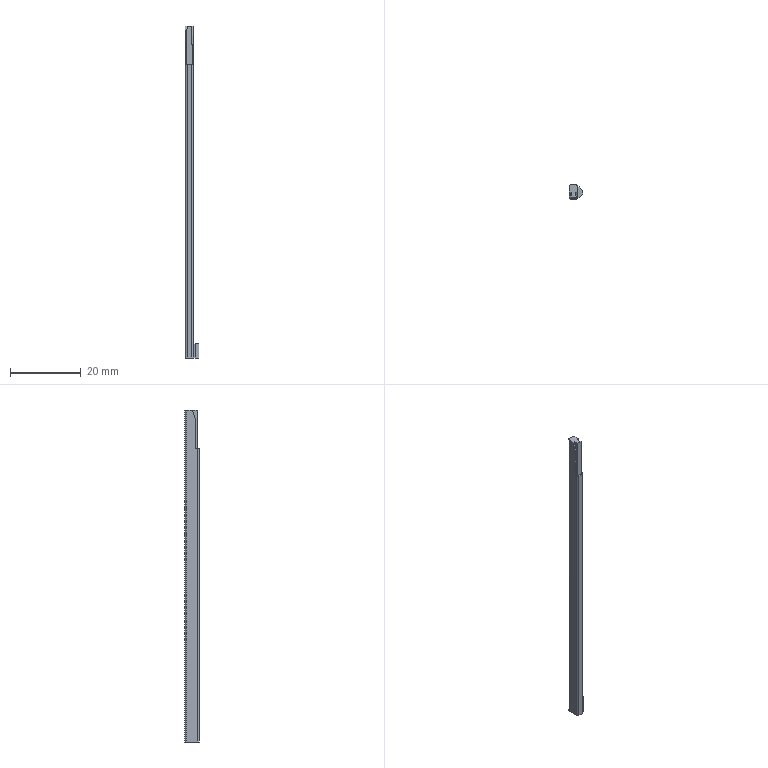Part | Creo | 1 solid | 24 faces | box 3.8 x 3.995 x 94.171 mm | volume 844.433 mm3 | plane 20 | cylinder 4 | commonest cylinder face diameters 1 x4
STEP:
#1=CARTESIAN_POINT('',(0.,0.,0.));
#2=DIRECTION('',(0.,0.,1.));
#3=DIRECTION('',(1.,0.,0.));
#4=AXIS2_PLACEMENT_3D('',#1,#2,#3);
#5=CARTESIAN_POINT('',(-30.625,17.376,29.026));
#6=VERTEX_POINT('',#5);
#7=CARTESIAN_POINT('',(-30.625,17.448,37.282));
#8=VERTEX_POINT('',#7);
#9=CARTESIAN_POINT('',(-30.625,17.376,29.026));
#10=DIRECTION('',(0.,0.008727,1.));
#11=VECTOR('',#10,8.256);
#12=LINE('',#9,#11);
#13=EDGE_CURVE('',#6,#8,#12,.T.);
#14=ORIENTED_EDGE('',*,*,#13,.F.);
#15=CARTESIAN_POINT('',(-30.625,16.977,29.026));
#16=VERTEX_POINT('',#15);
#17=CARTESIAN_POINT('',(-30.625,17.376,29.026));
#18=DIRECTION('',(0.,-1.,0.));
#19=VECTOR('',#18,0.399);
#20=LINE('',#17,#19);
#21=EDGE_CURVE('',#6,#16,#20,.T.);
#22=ORIENTED_EDGE('',*,*,#21,.T.);
#23=CARTESIAN_POINT('',(-30.625,16.977,-54.09));
#24=VERTEX_POINT('',#23);
#25=CARTESIAN_POINT('',(-30.625,16.977,29.026));
#26=DIRECTION('',(0.,0.,-1.));
#27=VECTOR('',#26,83.116);
#28=LINE('',#25,#27);
#29=EDGE_CURVE('',#16,#24,#28,.T.);
#30=ORIENTED_EDGE('',*,*,#29,.T.);
#31=CARTESIAN_POINT('',(-30.625,19.972,-54.09));
#32=VERTEX_POINT('',#31);
#33=CARTESIAN_POINT('',(-30.625,16.977,-54.09));
#34=DIRECTION('',(0.,1.,0.));
#35=VECTOR('',#34,2.995);
#36=LINE('',#33,#35);
#37=EDGE_CURVE('',#24,#32,#36,.T.);
#38=ORIENTED_EDGE('',*,*,#37,.T.);
#39=CARTESIAN_POINT('',(-30.625,19.972,40.081));
#40=VERTEX_POINT('',#39);
#41=CARTESIAN_POINT('',(-30.625,19.972,-54.09));
#42=DIRECTION('',(0.,0.,1.));
#43=VECTOR('',#42,94.171);
#44=LINE('',#41,#43);
#45=EDGE_CURVE('',#32,#40,#44,.T.);
#46=ORIENTED_EDGE('',*,*,#45,.T.);
#47=CARTESIAN_POINT('',(-30.625,18.381,40.081));
#48=VERTEX_POINT('',#47);
#49=CARTESIAN_POINT('',(-30.625,18.381,40.081));
#50=DIRECTION('',(0.,1.,0.));
#51=VECTOR('',#50,1.591);
#52=LINE('',#49,#51);
#53=EDGE_CURVE('',#48,#40,#52,.T.);
#54=ORIENTED_EDGE('',*,*,#53,.F.);
#55=CARTESIAN_POINT('',(-30.625,17.448,37.282));
#56=DIRECTION('',(0.,0.3162,0.9487));
#57=VECTOR('',#56,2.95);
#58=LINE('',#55,#57);
#59=EDGE_CURVE('',#8,#48,#58,.T.);
#60=ORIENTED_EDGE('',*,*,#59,.F.);
#61=EDGE_LOOP('',(#14,#22,#30,#38,#46,#54,#60));
#62=FACE_OUTER_BOUND('',#61,.F.);
#63=CARTESIAN_POINT('',(-30.625,18.475,-145.974));
#64=DIRECTION('',(-1.,0.,0.));
#65=DIRECTION('',(0.,0.,1.));
#66=AXIS2_PLACEMENT_3D('',#63,#64,#65);
#67=PLANE('',#66);
#68=ADVANCED_FACE('',(#62),#67,.T.);
#69=CARTESIAN_POINT('',(-30.181,17.448,37.282));
#70=VERTEX_POINT('',#69);
#71=CARTESIAN_POINT('',(-30.181,17.448,37.282));
#72=DIRECTION('',(-1.,0.,0.));
#73=VECTOR('',#72,0.4441);
#74=LINE('',#71,#73);
#75=EDGE_CURVE('',#70,#8,#74,.T.);
#76=ORIENTED_EDGE('',*,*,#75,.F.);
#77=CARTESIAN_POINT('',(-30.325,17.376,29.026));
#78=VERTEX_POINT('',#77);
#79=CARTESIAN_POINT('',(-30.181,17.448,37.282));
#80=DIRECTION('',(-0.01745,-0.008725,-0.9998));
#81=VECTOR('',#80,8.258);
#82=LINE('',#79,#81);
#83=EDGE_CURVE('',#70,#78,#82,.T.);
#84=ORIENTED_EDGE('',*,*,#83,.T.);
#85=CARTESIAN_POINT('',(-30.625,17.376,29.026));
#86=DIRECTION('',(1.,0.,0.));
#87=VECTOR('',#86,0.3);
#88=LINE('',#85,#87);
#89=EDGE_CURVE('',#6,#78,#88,.T.);
#90=ORIENTED_EDGE('',*,*,#89,.F.);
#91=ORIENTED_EDGE('',*,*,#13,.T.);
#92=EDGE_LOOP('',(#76,#84,#90,#91));
#93=FACE_OUTER_BOUND('',#92,.F.);
#94=CARTESIAN_POINT('',(-34.848,17.376,29.026));
#95=DIRECTION('',(0.,1.,-0.008727));
#96=DIRECTION('',(-1.,0.,0.));
#97=AXIS2_PLACEMENT_3D('',#94,#95,#96);
#98=PLANE('',#97);
#99=ADVANCED_FACE('',(#93),#98,.F.);
#100=ORIENTED_EDGE('',*,*,#75,.T.);
#101=ORIENTED_EDGE('',*,*,#59,.T.);
#102=CARTESIAN_POINT('',(-30.132,18.381,40.081));
#103=VERTEX_POINT('',#102);
#104=CARTESIAN_POINT('',(-30.132,18.381,40.081));
#105=DIRECTION('',(-1.,0.,0.));
#106=VECTOR('',#105,0.493);
#107=LINE('',#104,#106);
#108=EDGE_CURVE('',#103,#48,#107,.T.);
#109=ORIENTED_EDGE('',*,*,#108,.F.);
#110=CARTESIAN_POINT('',(-30.132,18.381,40.081));
#111=DIRECTION('',(-0.01656,-0.3162,-0.9486));
#112=VECTOR('',#111,2.951);
#113=LINE('',#110,#112);
#114=EDGE_CURVE('',#103,#70,#113,.T.);
#115=ORIENTED_EDGE('',*,*,#114,.T.);
#116=EDGE_LOOP('',(#100,#101,#109,#115));
#117=FACE_OUTER_BOUND('',#116,.F.);
#118=CARTESIAN_POINT('',(-31.682,18.381,40.081));
#119=DIRECTION('',(0.,-0.9487,0.3162));
#120=DIRECTION('',(0.,-0.3162,-0.9487));
#121=AXIS2_PLACEMENT_3D('',#118,#119,#120);
#122=PLANE('',#121);
#123=ADVANCED_FACE('',(#117),#122,.T.);
#124=ORIENTED_EDGE('',*,*,#108,.T.);
#125=ORIENTED_EDGE('',*,*,#53,.T.);
#126=CARTESIAN_POINT('',(-30.125,20.472,40.081));
#127=VERTEX_POINT('',#126);
#128=CARTESIAN_POINT('',(-30.125,19.972,40.081));
#129=DIRECTION('',(0.,0.,1.));
#130=DIRECTION('',(0.,1.,0.));
#131=AXIS2_PLACEMENT_3D('',#128,#129,#130);
#132=CIRCLE('',#131,0.5);
#133=EDGE_CURVE('',#127,#40,#132,.T.);
#134=ORIENTED_EDGE('',*,*,#133,.F.);
#135=CARTESIAN_POINT('',(-28.824,20.472,40.081));
#136=VERTEX_POINT('',#135);
#137=CARTESIAN_POINT('',(-30.125,20.472,40.081));
#138=DIRECTION('',(1.,0.,0.));
#139=VECTOR('',#138,1.3);
#140=LINE('',#137,#139);
#141=EDGE_CURVE('',#127,#136,#140,.T.);
#142=ORIENTED_EDGE('',*,*,#141,.T.);
#143=CARTESIAN_POINT('',(-28.324,19.972,40.081));
#144=VERTEX_POINT('',#143);
#145=CARTESIAN_POINT('',(-28.824,19.972,40.081));
#146=DIRECTION('',(0.,0.,1.));
#147=DIRECTION('',(1.,0.,0.));
#148=AXIS2_PLACEMENT_3D('',#145,#146,#147);
#149=CIRCLE('',#148,0.5);
#150=EDGE_CURVE('',#144,#136,#149,.T.);
#151=ORIENTED_EDGE('',*,*,#150,.F.);
#152=CARTESIAN_POINT('',(-28.324,18.381,40.081));
#153=VERTEX_POINT('',#152);
#154=CARTESIAN_POINT('',(-28.324,19.972,40.081));
#155=DIRECTION('',(0.,-1.,0.));
#156=VECTOR('',#155,1.591);
#157=LINE('',#154,#156);
#158=EDGE_CURVE('',#144,#153,#157,.T.);
#159=ORIENTED_EDGE('',*,*,#158,.T.);
#160=CARTESIAN_POINT('',(-28.817,18.381,40.081));
#161=VERTEX_POINT('',#160);
#162=CARTESIAN_POINT('',(-28.817,18.381,40.081));
#163=DIRECTION('',(1.,0.,0.));
#164=VECTOR('',#163,0.493);
#165=LINE('',#162,#164);
#166=EDGE_CURVE('',#161,#153,#165,.T.);
#167=ORIENTED_EDGE('',*,*,#166,.F.);
#168=CARTESIAN_POINT('',(-28.817,16.97,40.081));
#169=VERTEX_POINT('',#168);
#170=CARTESIAN_POINT('',(-28.817,16.97,40.081));
#171=DIRECTION('',(0.,1.,0.));
#172=VECTOR('',#171,1.411);
#173=LINE('',#170,#172);
#174=EDGE_CURVE('',#169,#161,#173,.T.);
#175=ORIENTED_EDGE('',*,*,#174,.F.);
#176=CARTESIAN_POINT('',(-30.132,16.97,40.081));
#177=VERTEX_POINT('',#176);
#178=CARTESIAN_POINT('',(-30.132,16.97,40.081));
#179=DIRECTION('',(1.,0.,0.));
#180=VECTOR('',#179,1.315);
#181=LINE('',#178,#180);
#182=EDGE_CURVE('',#177,#169,#181,.T.);
#183=ORIENTED_EDGE('',*,*,#182,.F.);
#184=CARTESIAN_POINT('',(-30.132,18.381,40.081));
#185=DIRECTION('',(0.,-1.,0.));
#186=VECTOR('',#185,1.411);
#187=LINE('',#184,#186);
#188=EDGE_CURVE('',#103,#177,#187,.T.);
#189=ORIENTED_EDGE('',*,*,#188,.F.);
#190=EDGE_LOOP('',(#124,#125,#134,#142,#151,#159,#167,#175,#183,#189));
#191=FACE_OUTER_BOUND('',#190,.F.);
#192=CARTESIAN_POINT('',(-17.817,-88.35,40.081));
#193=DIRECTION('',(0.,0.,1.));
#194=DIRECTION('',(-1.,0.,0.));
#195=AXIS2_PLACEMENT_3D('',#192,#193,#194);
#196=PLANE('',#195);
#197=ADVANCED_FACE('',(#191),#196,.T.);
#198=ORIENTED_EDGE('',*,*,#133,.T.);
#199=ORIENTED_EDGE('',*,*,#45,.F.);
#200=CARTESIAN_POINT('',(-30.125,20.472,-54.09));
#201=VERTEX_POINT('',#200);
#202=CARTESIAN_POINT('',(-30.125,19.972,-54.09));
#203=DIRECTION('',(0.,0.,-1.));
#204=DIRECTION('',(-1.,0.,0.));
#205=AXIS2_PLACEMENT_3D('',#202,#203,#204);
#206=CIRCLE('',#205,0.5);
#207=EDGE_CURVE('',#32,#201,#206,.T.);
#208=ORIENTED_EDGE('',*,*,#207,.T.);
#209=CARTESIAN_POINT('',(-30.125,20.472,40.081));
#210=DIRECTION('',(0.,0.,-1.));
#211=VECTOR('',#210,94.171);
#212=LINE('',#209,#211);
#213=EDGE_CURVE('',#127,#201,#212,.T.);
#214=ORIENTED_EDGE('',*,*,#213,.F.);
#215=EDGE_LOOP('',(#198,#199,#208,#214));
#216=FACE_OUTER_BOUND('',#215,.F.);
#217=CARTESIAN_POINT('',(-30.125,19.972,-145.974));
#218=DIRECTION('',(0.,0.,1.));
#219=DIRECTION('',(1.,0.,0.));
#220=AXIS2_PLACEMENT_3D('',#217,#218,#219);
#221=CYLINDRICAL_SURFACE('',#220,0.5);
#222=ADVANCED_FACE('',(#216),#221,.T.);
#223=CARTESIAN_POINT('',(-26.824,18.972,-54.09));
#224=VERTEX_POINT('',#223);
#225=CARTESIAN_POINT('',(-26.824,17.977,-54.09));
#226=VERTEX_POINT('',#225);
#227=CARTESIAN_POINT('',(-26.824,18.972,-54.09));
#228=DIRECTION('',(0.,-1.,0.));
#229=VECTOR('',#228,0.9955);
#230=LINE('',#227,#229);
#231=EDGE_CURVE('',#224,#226,#230,.T.);
#232=ORIENTED_EDGE('',*,*,#231,.F.);
#233=CARTESIAN_POINT('',(-27.824,19.972,-54.09));
#234=VERTEX_POINT('',#233);
#235=CARTESIAN_POINT('',(-27.824,19.972,-54.09));
#236=DIRECTION('',(0.7071,-0.7071,0.));
#237=VECTOR('',#236,1.414);
#238=LINE('',#235,#237);
#239=EDGE_CURVE('',#234,#224,#238,.T.);
#240=ORIENTED_EDGE('',*,*,#239,.F.);
#241=CARTESIAN_POINT('',(-28.324,19.972,-54.09));
#242=VERTEX_POINT('',#241);
#243=CARTESIAN_POINT('',(-28.324,19.972,-54.09));
#244=DIRECTION('',(1.,0.,0.));
#245=VECTOR('',#244,0.5);
#246=LINE('',#243,#245);
#247=EDGE_CURVE('',#242,#234,#246,.T.);
#248=ORIENTED_EDGE('',*,*,#247,.F.);
#249=CARTESIAN_POINT('',(-28.824,20.472,-54.09));
#250=VERTEX_POINT('',#249);
#251=CARTESIAN_POINT('',(-28.824,19.972,-54.09));
#252=DIRECTION('',(0.,0.,-1.));
#253=DIRECTION('',(0.,1.,0.));
#254=AXIS2_PLACEMENT_3D('',#251,#252,#253);
#255=CIRCLE('',#254,0.5);
#256=EDGE_CURVE('',#250,#242,#255,.T.);
#257=ORIENTED_EDGE('',*,*,#256,.F.);
#258=CARTESIAN_POINT('',(-30.125,20.472,-54.09));
#259=DIRECTION('',(1.,0.,0.));
#260=VECTOR('',#259,1.3);
#261=LINE('',#258,#260);
#262=EDGE_CURVE('',#201,#250,#261,.T.);
#263=ORIENTED_EDGE('',*,*,#262,.F.);
#264=ORIENTED_EDGE('',*,*,#207,.F.);
#265=ORIENTED_EDGE('',*,*,#37,.F.);
#266=CARTESIAN_POINT('',(-30.125,16.477,-54.09));
#267=VERTEX_POINT('',#266);
#268=CARTESIAN_POINT('',(-30.125,16.977,-54.09));
#269=DIRECTION('',(0.,0.,-1.));
#270=DIRECTION('',(0.,-1.,0.));
#271=AXIS2_PLACEMENT_3D('',#268,#269,#270);
#272=CIRCLE('',#271,0.5);
#273=EDGE_CURVE('',#267,#24,#272,.T.);
#274=ORIENTED_EDGE('',*,*,#273,.F.);
#275=CARTESIAN_POINT('',(-28.824,16.477,-54.09));
#276=VERTEX_POINT('',#275);
#277=CARTESIAN_POINT('',(-28.824,16.477,-54.09));
#278=DIRECTION('',(-1.,0.,0.));
#279=VECTOR('',#278,1.3);
#280=LINE('',#277,#279);
#281=EDGE_CURVE('',#276,#267,#280,.T.);
#282=ORIENTED_EDGE('',*,*,#281,.F.);
#283=CARTESIAN_POINT('',(-28.324,16.977,-54.09));
#284=VERTEX_POINT('',#283);
#285=CARTESIAN_POINT('',(-28.824,16.977,-54.09));
#286=DIRECTION('',(0.,0.,-1.));
#287=DIRECTION('',(1.,0.,0.));
#288=AXIS2_PLACEMENT_3D('',#285,#286,#287);
#289=CIRCLE('',#288,0.5);
#290=EDGE_CURVE('',#284,#276,#289,.T.);
#291=ORIENTED_EDGE('',*,*,#290,.F.);
#292=CARTESIAN_POINT('',(-27.824,16.977,-54.09));
#293=VERTEX_POINT('',#292);
#294=CARTESIAN_POINT('',(-27.824,16.977,-54.09));
#295=DIRECTION('',(-1.,0.,0.));
#296=VECTOR('',#295,0.5);
#297=LINE('',#294,#296);
#298=EDGE_CURVE('',#293,#284,#297,.T.);
#299=ORIENTED_EDGE('',*,*,#298,.F.);
#300=CARTESIAN_POINT('',(-26.824,17.977,-54.09));
#301=DIRECTION('',(-0.7071,-0.7071,0.));
#302=VECTOR('',#301,1.414);
#303=LINE('',#300,#302);
#304=EDGE_CURVE('',#226,#293,#303,.T.);
#305=ORIENTED_EDGE('',*,*,#304,.F.);
#306=EDGE_LOOP('',(#232,#240,#248,#257,#263,#264,#265,#274,#282,#291,#299,#305));
#307=FACE_OUTER_BOUND('',#306,.F.);
#308=CARTESIAN_POINT('',(0.,0.,-54.09));
#309=DIRECTION('',(0.,0.,-1.));
#310=DIRECTION('',(-1.,0.,0.));
#311=AXIS2_PLACEMENT_3D('',#308,#309,#310);
#312=PLANE('',#311);
#313=ADVANCED_FACE('',(#307),#312,.T.);
#314=CARTESIAN_POINT('',(-26.824,17.977,-50.09));
#315=VERTEX_POINT('',#314);
#316=CARTESIAN_POINT('',(-26.824,18.972,-50.09));
#317=VERTEX_POINT('',#316);
#318=CARTESIAN_POINT('',(-26.824,17.977,-50.09));
#319=DIRECTION('',(0.,1.,0.));
#320=VECTOR('',#319,0.9955);
#321=LINE('',#318,#320);
#322=EDGE_CURVE('',#315,#317,#321,.T.);
#323=ORIENTED_EDGE('',*,*,#322,.T.);
#324=CARTESIAN_POINT('',(-26.824,18.972,-50.09));
#325=DIRECTION('',(0.,0.,-1.));
#326=VECTOR('',#325,4.);
#327=LINE('',#324,#326);
#328=EDGE_CURVE('',#317,#224,#327,.T.);
#329=ORIENTED_EDGE('',*,*,#328,.T.);
#330=ORIENTED_EDGE('',*,*,#231,.T.);
#331=CARTESIAN_POINT('',(-26.824,17.977,-54.09));
#332=DIRECTION('',(0.,0.,1.));
#333=VECTOR('',#332,4.);
#334=LINE('',#331,#333);
#335=EDGE_CURVE('',#226,#315,#334,.T.);
#336=ORIENTED_EDGE('',*,*,#335,.T.);
#337=EDGE_LOOP('',(#323,#329,#330,#336));
#338=FACE_OUTER_BOUND('',#337,.F.);
#339=CARTESIAN_POINT('',(-26.824,18.475,-54.09));
#340=DIRECTION('',(1.,0.,0.));
#341=DIRECTION('',(0.,0.,-1.));
#342=AXIS2_PLACEMENT_3D('',#339,#340,#341);
#343=PLANE('',#342);
#344=ADVANCED_FACE('',(#338),#343,.T.);
#345=CARTESIAN_POINT('',(-28.324,16.977,-50.09));
#346=VERTEX_POINT('',#345);
#347=CARTESIAN_POINT('',(-27.824,16.977,-50.09));
#348=VERTEX_POINT('',#347);
#349=CARTESIAN_POINT('',(-28.324,16.977,-50.09));
#350=DIRECTION('',(1.,0.,0.));
#351=VECTOR('',#350,0.5);
#352=LINE('',#349,#351);
#353=EDGE_CURVE('',#346,#348,#352,.T.);
#354=ORIENTED_EDGE('',*,*,#353,.F.);
#355=CARTESIAN_POINT('',(-28.324,19.972,-50.09));
#356=VERTEX_POINT('',#355);
#357=CARTESIAN_POINT('',(-28.324,16.977,-50.09));
#358=DIRECTION('',(0.,1.,0.));
#359=VECTOR('',#358,2.995);
#360=LINE('',#357,#359);
#361=EDGE_CURVE('',#346,#356,#360,.T.);
#362=ORIENTED_EDGE('',*,*,#361,.T.);
#363=CARTESIAN_POINT('',(-27.824,19.972,-50.09));
#364=VERTEX_POINT('',#363);
#365=CARTESIAN_POINT('',(-27.824,19.972,-50.09));
#366=DIRECTION('',(-1.,0.,0.));
#367=VECTOR('',#366,0.5);
#368=LINE('',#365,#367);
#369=EDGE_CURVE('',#364,#356,#368,.T.);
#370=ORIENTED_EDGE('',*,*,#369,.F.);
#371=CARTESIAN_POINT('',(-26.824,18.972,-50.09));
#372=DIRECTION('',(-0.7071,0.7071,0.));
#373=VECTOR('',#372,1.414);
#374=LINE('',#371,#373);
#375=EDGE_CURVE('',#317,#364,#374,.T.);
#376=ORIENTED_EDGE('',*,*,#375,.F.);
#377=ORIENTED_EDGE('',*,*,#322,.F.);
#378=CARTESIAN_POINT('',(-27.824,16.977,-50.09));
#379=DIRECTION('',(0.7071,0.7071,0.));
#380=VECTOR('',#379,1.414);
#381=LINE('',#378,#380);
#382=EDGE_CURVE('',#348,#315,#381,.T.);
#383=ORIENTED_EDGE('',*,*,#382,.F.);
#384=EDGE_LOOP('',(#354,#362,#370,#376,#377,#383));
#385=FACE_OUTER_BOUND('',#384,.F.);
#386=CARTESIAN_POINT('',(-28.074,18.475,-50.09));
#387=DIRECTION('',(0.,0.,1.));
#388=DIRECTION('',(1.,0.,0.));
#389=AXIS2_PLACEMENT_3D('',#386,#387,#388);
#390=PLANE('',#389);
#391=ADVANCED_FACE('',(#385),#390,.T.);
#392=ORIENTED_EDGE('',*,*,#298,.T.);
#393=CARTESIAN_POINT('',(-28.324,16.977,-54.09));
#394=DIRECTION('',(0.,0.,1.));
#395=VECTOR('',#394,4.);
#396=LINE('',#393,#395);
#397=EDGE_CURVE('',#284,#346,#396,.T.);
#398=ORIENTED_EDGE('',*,*,#397,.T.);
#399=ORIENTED_EDGE('',*,*,#353,.T.);
#400=CARTESIAN_POINT('',(-27.824,16.977,-50.09));
#401=DIRECTION('',(0.,0.,-1.));
#402=VECTOR('',#401,4.);
#403=LINE('',#400,#402);
#404=EDGE_CURVE('',#348,#293,#403,.T.);
#405=ORIENTED_EDGE('',*,*,#404,.T.);
#406=EDGE_LOOP('',(#392,#398,#399,#405));
#407=FACE_OUTER_BOUND('',#406,.F.);
#408=CARTESIAN_POINT('',(-28.074,16.977,-54.09));
#409=DIRECTION('',(0.,-1.,0.));
#410=DIRECTION('',(0.,0.,-1.));
#411=AXIS2_PLACEMENT_3D('',#408,#409,#410);
#412=PLANE('',#411);
#413=ADVANCED_FACE('',(#407),#412,.T.);
#414=CARTESIAN_POINT('',(-28.324,16.977,29.026));
#415=VERTEX_POINT('',#414);
#416=CARTESIAN_POINT('',(-28.324,16.977,-50.09));
#417=DIRECTION('',(0.,0.,1.));
#418=VECTOR('',#417,79.116);
#419=LINE('',#416,#418);
#420=EDGE_CURVE('',#346,#415,#419,.T.);
#421=ORIENTED_EDGE('',*,*,#420,.F.);
#422=ORIENTED_EDGE('',*,*,#397,.F.);
#423=ORIENTED_EDGE('',*,*,#290,.T.);
#424=CARTESIAN_POINT('',(-28.824,16.477,29.026));
#425=VERTEX_POINT('',#424);
#426=CARTESIAN_POINT('',(-28.824,16.477,29.026));
#427=DIRECTION('',(0.,0.,-1.));
#428=VECTOR('',#427,83.116);
#429=LINE('',#426,#428);
#430=EDGE_CURVE('',#425,#276,#429,.T.);
#431=ORIENTED_EDGE('',*,*,#430,.F.);
#432=CARTESIAN_POINT('',(-28.824,16.977,29.026));
#433=DIRECTION('',(0.,0.,1.));
#434=DIRECTION('',(0.,-1.,0.));
#435=AXIS2_PLACEMENT_3D('',#432,#433,#434);
#436=CIRCLE('',#435,0.5);
#437=EDGE_CURVE('',#425,#415,#436,.T.);
#438=ORIENTED_EDGE('',*,*,#437,.T.);
#439=EDGE_LOOP('',(#421,#422,#423,#431,#438));
#440=FACE_OUTER_BOUND('',#439,.F.);
#441=CARTESIAN_POINT('',(-28.824,16.977,-145.974));
#442=DIRECTION('',(0.,0.,1.));
#443=DIRECTION('',(1.,0.,0.));
#444=AXIS2_PLACEMENT_3D('',#441,#442,#443);
#445=CYLINDRICAL_SURFACE('',#444,0.5);
#446=ADVANCED_FACE('',(#440),#445,.T.);
#447=CARTESIAN_POINT('',(-28.324,17.448,37.282));
#448=VERTEX_POINT('',#447);
#449=CARTESIAN_POINT('',(-28.324,18.381,40.081));
#450=DIRECTION('',(0.,-0.3162,-0.9487));
#451=VECTOR('',#450,2.95);
#452=LINE('',#449,#451);
#453=EDGE_CURVE('',#153,#448,#452,.T.);
#454=ORIENTED_EDGE('',*,*,#453,.F.);
#455=ORIENTED_EDGE('',*,*,#158,.F.);
#456=CARTESIAN_POINT('',(-28.324,19.972,40.081));
#457=DIRECTION('',(0.,0.,-1.));
#458=VECTOR('',#457,90.171);
#459=LINE('',#456,#458);
#460=EDGE_CURVE('',#144,#356,#459,.T.);
#461=ORIENTED_EDGE('',*,*,#460,.T.);
#462=ORIENTED_EDGE('',*,*,#361,.F.);
#463=ORIENTED_EDGE('',*,*,#420,.T.);
#464=CARTESIAN_POINT('',(-28.324,17.376,29.026));
#465=VERTEX_POINT('',#464);
#466=CARTESIAN_POINT('',(-28.324,16.977,29.026));
#467=DIRECTION('',(0.,1.,0.));
#468=VECTOR('',#467,0.399);
#469=LINE('',#466,#468);
#470=EDGE_CURVE('',#415,#465,#469,.T.);
#471=ORIENTED_EDGE('',*,*,#470,.T.);
#472=CARTESIAN_POINT('',(-28.324,17.448,37.282));
#473=DIRECTION('',(0.,-0.008727,-1.));
#474=VECTOR('',#473,8.256);
#475=LINE('',#472,#474);
#476=EDGE_CURVE('',#448,#465,#475,.T.);
#477=ORIENTED_EDGE('',*,*,#476,.F.);
#478=EDGE_LOOP('',(#454,#455,#461,#462,#463,#471,#477));
#479=FACE_OUTER_BOUND('',#478,.F.);
#480=CARTESIAN_POINT('',(-28.324,18.475,-145.974));
#481=DIRECTION('',(1.,0.,0.));
#482=DIRECTION('',(0.,0.,-1.));
#483=AXIS2_PLACEMENT_3D('',#480,#481,#482);
#484=PLANE('',#483);
#485=ADVANCED_FACE('',(#479),#484,.T.);
#486=ORIENTED_EDGE('',*,*,#453,.T.);
#487=CARTESIAN_POINT('',(-28.768,17.448,37.282));
#488=VERTEX_POINT('',#487);
#489=CARTESIAN_POINT('',(-28.768,17.448,37.282));
#490=DIRECTION('',(1.,0.,0.));
#491=VECTOR('',#490,0.4441);
#492=LINE('',#489,#491);
#493=EDGE_CURVE('',#488,#448,#492,.T.);
#494=ORIENTED_EDGE('',*,*,#493,.F.);
#495=CARTESIAN_POINT('',(-28.817,18.381,40.081));
#496=DIRECTION('',(0.01656,-0.3162,-0.9486));
#497=VECTOR('',#496,2.951);
#498=LINE('',#495,#497);
#499=EDGE_CURVE('',#161,#488,#498,.T.);
#500=ORIENTED_EDGE('',*,*,#499,.F.);
#501=ORIENTED_EDGE('',*,*,#166,.T.);
#502=EDGE_LOOP('',(#486,#494,#500,#501));
#503=FACE_OUTER_BOUND('',#502,.F.);
#504=CARTESIAN_POINT('',(-27.267,18.381,40.081));
#505=DIRECTION('',(0.,0.9487,-0.3162));
#506=DIRECTION('',(0.,0.3162,0.9487));
#507=AXIS2_PLACEMENT_3D('',#504,#505,#506);
#508=PLANE('',#507);
#509=ADVANCED_FACE('',(#503),#508,.F.);
#510=CARTESIAN_POINT('',(-28.624,17.376,29.026));
#511=VERTEX_POINT('',#510);
#512=CARTESIAN_POINT('',(-28.624,17.376,29.026));
#513=DIRECTION('',(1.,0.,0.));
#514=VECTOR('',#513,0.3);
#515=LINE('',#512,#514);
#516=EDGE_CURVE('',#511,#465,#515,.T.);
#517=ORIENTED_EDGE('',*,*,#516,.F.);
#518=CARTESIAN_POINT('',(-28.768,17.448,37.282));
#519=DIRECTION('',(0.01745,-0.008725,-0.9998));
#520=VECTOR('',#519,8.258);
#521=LINE('',#518,#520);
#522=EDGE_CURVE('',#488,#511,#521,.T.);
#523=ORIENTED_EDGE('',*,*,#522,.F.);
#524=ORIENTED_EDGE('',*,*,#493,.T.);
#525=ORIENTED_EDGE('',*,*,#476,.T.);
#526=EDGE_LOOP('',(#517,#523,#524,#525));
#527=FACE_OUTER_BOUND('',#526,.F.);
#528=CARTESIAN_POINT('',(-32.335,17.376,29.026));
#529=DIRECTION('',(0.,1.,-0.008727));
#530=DIRECTION('',(-1.,0.,0.));
#531=AXIS2_PLACEMENT_3D('',#528,#529,#530);
#532=PLANE('',#531);
#533=ADVANCED_FACE('',(#527),#532,.F.);
#534=ORIENTED_EDGE('',*,*,#21,.F.);
#535=ORIENTED_EDGE('',*,*,#89,.T.);
#536=CARTESIAN_POINT('',(-30.325,16.777,29.026));
#537=VERTEX_POINT('',#536);
#538=CARTESIAN_POINT('',(-30.325,17.376,29.026));
#539=DIRECTION('',(0.,-1.,0.));
#540=VECTOR('',#539,0.599);
#541=LINE('',#538,#540);
#542=EDGE_CURVE('',#78,#537,#541,.T.);
#543=ORIENTED_EDGE('',*,*,#542,.T.);
#544=CARTESIAN_POINT('',(-28.624,16.777,29.026));
#545=VERTEX_POINT('',#544);
#546=CARTESIAN_POINT('',(-30.325,16.777,29.026));
#547=DIRECTION('',(1.,0.,0.));
#548=VECTOR('',#547,1.7);
#549=LINE('',#546,#548);
#550=EDGE_CURVE('',#537,#545,#549,.T.);
#551=ORIENTED_EDGE('',*,*,#550,.T.);
#552=CARTESIAN_POINT('',(-28.624,16.777,29.026));
#553=DIRECTION('',(0.,1.,0.));
#554=VECTOR('',#553,0.599);
#555=LINE('',#552,#554);
#556=EDGE_CURVE('',#545,#511,#555,.T.);
#557=ORIENTED_EDGE('',*,*,#556,.T.);
#558=ORIENTED_EDGE('',*,*,#516,.T.);
#559=ORIENTED_EDGE('',*,*,#470,.F.);
#560=ORIENTED_EDGE('',*,*,#437,.F.);
#561=CARTESIAN_POINT('',(-30.125,16.477,29.026));
#562=VERTEX_POINT('',#561);
#563=CARTESIAN_POINT('',(-30.125,16.477,29.026));
#564=DIRECTION('',(1.,0.,0.));
#565=VECTOR('',#564,1.3);
#566=LINE('',#563,#565);
#567=EDGE_CURVE('',#562,#425,#566,.T.);
#568=ORIENTED_EDGE('',*,*,#567,.F.);
#569=CARTESIAN_POINT('',(-30.125,16.977,29.026));
#570=DIRECTION('',(0.,0.,1.));
#571=DIRECTION('',(-1.,0.,0.));
#572=AXIS2_PLACEMENT_3D('',#569,#570,#571);
#573=CIRCLE('',#572,0.5);
#574=EDGE_CURVE('',#16,#562,#573,.T.);
#575=ORIENTED_EDGE('',*,*,#574,.F.);
#576=EDGE_LOOP('',(#534,#535,#543,#551,#557,#558,#559,#560,#568,#575));
#577=FACE_OUTER_BOUND('',#576,.F.);
#578=CARTESIAN_POINT('',(-0.07825,-88.35,29.026));
#579=DIRECTION('',(0.,0.,-1.));
#580=DIRECTION('',(0.,-1.,0.));
#581=AXIS2_PLACEMENT_3D('',#578,#579,#580);
#582=PLANE('',#581);
#583=ADVANCED_FACE('',(#577),#582,.F.);
#584=ORIENTED_EDGE('',*,*,#114,.F.);
#585=ORIENTED_EDGE('',*,*,#188,.T.);
#586=CARTESIAN_POINT('',(-30.132,16.97,40.081));
#587=DIRECTION('',(-0.01745,-0.01745,-0.9997));
#588=VECTOR('',#587,11.058);
#589=LINE('',#586,#588);
#590=EDGE_CURVE('',#177,#537,#589,.T.);
#591=ORIENTED_EDGE('',*,*,#590,.T.);
#592=ORIENTED_EDGE('',*,*,#542,.F.);
#593=ORIENTED_EDGE('',*,*,#83,.F.);
#594=EDGE_LOOP('',(#584,#585,#591,#592,#593));
#595=FACE_OUTER_BOUND('',#594,.F.);
#596=CARTESIAN_POINT('',(-30.132,17.472,40.081));
#597=DIRECTION('',(0.9998,0.,-0.01745));
#598=DIRECTION('',(-0.01745,0.,-0.9998));
#599=AXIS2_PLACEMENT_3D('',#596,#597,#598);
#600=PLANE('',#599);
#601=ADVANCED_FACE('',(#595),#600,.F.);
#602=ORIENTED_EDGE('',*,*,#550,.F.);
#603=ORIENTED_EDGE('',*,*,#590,.F.);
#604=ORIENTED_EDGE('',*,*,#182,.T.);
#605=CARTESIAN_POINT('',(-28.817,16.97,40.081));
#606=DIRECTION('',(0.01745,-0.01745,-0.9997));
#607=VECTOR('',#606,11.058);
#608=LINE('',#605,#607);
#609=EDGE_CURVE('',#169,#545,#608,.T.);
#610=ORIENTED_EDGE('',*,*,#609,.T.);
#611=EDGE_LOOP('',(#602,#603,#604,#610));
#612=FACE_OUTER_BOUND('',#611,.F.);
#613=CARTESIAN_POINT('',(-30.132,16.97,40.081));
#614=DIRECTION('',(0.,0.9998,-0.01745));
#615=DIRECTION('',(0.,-0.01745,-0.9998));
#616=AXIS2_PLACEMENT_3D('',#613,#614,#615);
#617=PLANE('',#616);
#618=ADVANCED_FACE('',(#612),#617,.F.);
#619=ORIENTED_EDGE('',*,*,#522,.T.);
#620=ORIENTED_EDGE('',*,*,#556,.F.);
#621=ORIENTED_EDGE('',*,*,#609,.F.);
#622=ORIENTED_EDGE('',*,*,#174,.T.);
#623=ORIENTED_EDGE('',*,*,#499,.T.);
#624=EDGE_LOOP('',(#619,#620,#621,#622,#623));
#625=FACE_OUTER_BOUND('',#624,.F.);
#626=CARTESIAN_POINT('',(-28.817,16.97,40.081));
#627=DIRECTION('',(-0.9998,0.,-0.01745));
#628=DIRECTION('',(-0.01745,0.,0.9998));
#629=AXIS2_PLACEMENT_3D('',#626,#627,#628);
#630=PLANE('',#629);
#631=ADVANCED_FACE('',(#625),#630,.F.);
#632=ORIENTED_EDGE('',*,*,#430,.T.);
#633=ORIENTED_EDGE('',*,*,#281,.T.);
#634=CARTESIAN_POINT('',(-30.125,16.477,-54.09));
#635=DIRECTION('',(0.,0.,1.));
#636=VECTOR('',#635,83.116);
#637=LINE('',#634,#636);
#638=EDGE_CURVE('',#267,#562,#637,.T.);
#639=ORIENTED_EDGE('',*,*,#638,.T.);
#640=ORIENTED_EDGE('',*,*,#567,.T.);
#641=EDGE_LOOP('',(#632,#633,#639,#640));
#642=FACE_OUTER_BOUND('',#641,.F.);
#643=CARTESIAN_POINT('',(-29.474,16.477,-145.974));
#644=DIRECTION('',(0.,-1.,0.));
#645=DIRECTION('',(0.,0.,-1.));
#646=AXIS2_PLACEMENT_3D('',#643,#644,#645);
#647=PLANE('',#646);
#648=ADVANCED_FACE('',(#642),#647,.T.);
#649=ORIENTED_EDGE('',*,*,#638,.F.);
#650=ORIENTED_EDGE('',*,*,#273,.T.);
#651=ORIENTED_EDGE('',*,*,#29,.F.);
#652=ORIENTED_EDGE('',*,*,#574,.T.);
#653=EDGE_LOOP('',(#649,#650,#651,#652));
#654=FACE_OUTER_BOUND('',#653,.F.);
#655=CARTESIAN_POINT('',(-30.125,16.977,-145.974));
#656=DIRECTION('',(0.,0.,1.));
#657=DIRECTION('',(1.,0.,0.));
#658=AXIS2_PLACEMENT_3D('',#655,#656,#657);
#659=CYLINDRICAL_SURFACE('',#658,0.5);
#660=ADVANCED_FACE('',(#654),#659,.T.);
#661=ORIENTED_EDGE('',*,*,#150,.T.);
#662=CARTESIAN_POINT('',(-28.824,20.472,-54.09));
#663=DIRECTION('',(0.,0.,1.));
#664=VECTOR('',#663,94.171);
#665=LINE('',#662,#664);
#666=EDGE_CURVE('',#250,#136,#665,.T.);
#667=ORIENTED_EDGE('',*,*,#666,.F.);
#668=ORIENTED_EDGE('',*,*,#256,.T.);
#669=CARTESIAN_POINT('',(-28.324,19.972,-50.09));
#670=DIRECTION('',(0.,0.,-1.));
#671=VECTOR('',#670,4.);
#672=LINE('',#669,#671);
#673=EDGE_CURVE('',#356,#242,#672,.T.);
#674=ORIENTED_EDGE('',*,*,#673,.F.);
#675=ORIENTED_EDGE('',*,*,#460,.F.);
#676=EDGE_LOOP('',(#661,#667,#668,#674,#675));
#677=FACE_OUTER_BOUND('',#676,.F.);
#678=CARTESIAN_POINT('',(-28.824,19.972,-145.974));
#679=DIRECTION('',(0.,0.,1.));
#680=DIRECTION('',(1.,0.,0.));
#681=AXIS2_PLACEMENT_3D('',#678,#679,#680);
#682=CYLINDRICAL_SURFACE('',#681,0.5);
#683=ADVANCED_FACE('',(#677),#682,.T.);
#684=ORIENTED_EDGE('',*,*,#141,.F.);
#685=ORIENTED_EDGE('',*,*,#213,.T.);
#686=ORIENTED_EDGE('',*,*,#262,.T.);
#687=ORIENTED_EDGE('',*,*,#666,.T.);
#688=EDGE_LOOP('',(#684,#685,#686,#687));
#689=FACE_OUTER_BOUND('',#688,.F.);
#690=CARTESIAN_POINT('',(-29.474,20.472,-145.974));
#691=DIRECTION('',(0.,1.,0.));
#692=DIRECTION('',(0.,0.,1.));
#693=AXIS2_PLACEMENT_3D('',#690,#691,#692);
#694=PLANE('',#693);
#695=ADVANCED_FACE('',(#689),#694,.T.);
#696=ORIENTED_EDGE('',*,*,#369,.T.);
#697=ORIENTED_EDGE('',*,*,#673,.T.);
#698=ORIENTED_EDGE('',*,*,#247,.T.);
#699=CARTESIAN_POINT('',(-27.824,19.972,-54.09));
#700=DIRECTION('',(0.,0.,1.));
#701=VECTOR('',#700,4.);
#702=LINE('',#699,#701);
#703=EDGE_CURVE('',#234,#364,#702,.T.);
#704=ORIENTED_EDGE('',*,*,#703,.T.);
#705=EDGE_LOOP('',(#696,#697,#698,#704));
#706=FACE_OUTER_BOUND('',#705,.F.);
#707=CARTESIAN_POINT('',(-28.074,19.972,-54.09));
#708=DIRECTION('',(0.,1.,0.));
#709=DIRECTION('',(0.,0.,1.));
#710=AXIS2_PLACEMENT_3D('',#707,#708,#709);
#711=PLANE('',#710);
#712=ADVANCED_FACE('',(#706),#711,.T.);
#713=ORIENTED_EDGE('',*,*,#239,.T.);
#714=ORIENTED_EDGE('',*,*,#328,.F.);
#715=ORIENTED_EDGE('',*,*,#375,.T.);
#716=ORIENTED_EDGE('',*,*,#703,.F.);
#717=EDGE_LOOP('',(#713,#714,#715,#716));
#718=FACE_OUTER_BOUND('',#717,.F.);
#719=CARTESIAN_POINT('',(-26.824,18.972,-54.09));
#720=DIRECTION('',(-0.7071,-0.7071,0.));
#721=DIRECTION('',(0.,0.,1.));
#722=AXIS2_PLACEMENT_3D('',#719,#720,#721);
#723=PLANE('',#722);
#724=ADVANCED_FACE('',(#718),#723,.F.);
#725=ORIENTED_EDGE('',*,*,#304,.T.);
#726=ORIENTED_EDGE('',*,*,#404,.F.);
#727=ORIENTED_EDGE('',*,*,#382,.T.);
#728=ORIENTED_EDGE('',*,*,#335,.F.);
#729=EDGE_LOOP('',(#725,#726,#727,#728));
#730=FACE_OUTER_BOUND('',#729,.F.);
#731=CARTESIAN_POINT('',(-27.824,16.977,-54.09));
#732=DIRECTION('',(-0.7071,0.7071,0.));
#733=DIRECTION('',(0.,0.,1.));
#734=AXIS2_PLACEMENT_3D('',#731,#732,#733);
#735=PLANE('',#734);
#736=ADVANCED_FACE('',(#730),#735,.F.);
#737=CLOSED_SHELL('',(#68,#99,#123,#197,#222,#313,#344,#391,#413,#446,#485,#509,#533,#583,#601,#618,#631,#648,#660,#683,#695,#712,#724,#736));
#738=MANIFOLD_SOLID_BREP('',#737);
#739=(LENGTH_UNIT()NAMED_UNIT(*)SI_UNIT(.MILLI.,.METRE.));
#740=UNCERTAINTY_MEASURE_WITH_UNIT(LENGTH_MEASURE(0.009433),#739,'','');
#741=(NAMED_UNIT(*)PLANE_ANGLE_UNIT()SI_UNIT($,.RADIAN.));
#742=PLANE_ANGLE_MEASURE_WITH_UNIT(PLANE_ANGLE_MEASURE(0.01745),#741);
#743=(CONVERSION_BASED_UNIT('DEGREE',#742)NAMED_UNIT(*)PLANE_ANGLE_UNIT());
#744=(NAMED_UNIT(*)SI_UNIT($,.STERADIAN.)SOLID_ANGLE_UNIT());
#745=(GEOMETRIC_REPRESENTATION_CONTEXT(3)GLOBAL_UNCERTAINTY_ASSIGNED_CONTEXT((#740))GLOBAL_UNIT_ASSIGNED_CONTEXT((#739,#743,#744))REPRESENTATION_CONTEXT('',''));
#746=ADVANCED_BREP_SHAPE_REPRESENTATION('',(#4,#738),#745);